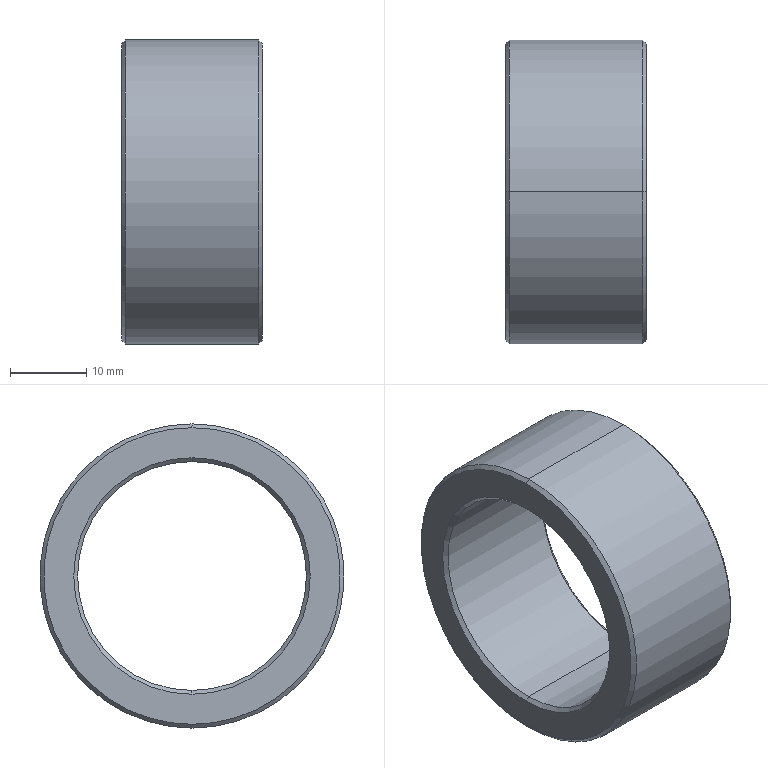Part | SolidWorks | features Chamfer 1, Extrusion 1 | 1 solid | 14 faces | box 18.5 x 40 x 40 mm | volume 10029 mm3 | cone 8 | cylinder 4 | plane 2 | commonest cylinder face diameters 30.1 x2 40 x2
STEP:
#1=CARTESIAN_POINT('',(18.5,0.,-19.5));
#2=VERTEX_POINT('',#1);
#3=CARTESIAN_POINT('',(18.5,0.,19.5));
#4=VERTEX_POINT('',#3);
#5=CARTESIAN_POINT('',(18.5,0.,0.));
#6=DIRECTION('',(1.,0.,0.));
#7=DIRECTION('',(0.,0.,-1.));
#8=AXIS2_PLACEMENT_3D('',#5,#6,#7);
#9=CIRCLE('',#8,19.5);
#10=EDGE_CURVE('',#2,#4,#9,.T.);
#11=ORIENTED_EDGE('',*,*,#10,.F.);
#12=CARTESIAN_POINT('',(18.,0.,-20.));
#13=VERTEX_POINT('',#12);
#14=CARTESIAN_POINT('',(18.5,0.,-19.5));
#15=DIRECTION('',(-0.7071,0.,-0.7071));
#16=VECTOR('',#15,1000.);
#17=LINE('',#14,#16);
#18=EDGE_CURVE('',#2,#13,#17,.T.);
#19=ORIENTED_EDGE('',*,*,#18,.T.);
#20=CARTESIAN_POINT('',(18.,0.,20.));
#21=VERTEX_POINT('',#20);
#22=CARTESIAN_POINT('',(18.,0.,0.));
#23=DIRECTION('',(-1.,0.,0.));
#24=DIRECTION('',(0.,0.,-1.));
#25=AXIS2_PLACEMENT_3D('',#22,#23,#24);
#26=CIRCLE('',#25,20.);
#27=EDGE_CURVE('',#21,#13,#26,.T.);
#28=ORIENTED_EDGE('',*,*,#27,.F.);
#29=CARTESIAN_POINT('',(18.5,0.,19.5));
#30=DIRECTION('',(-0.7071,0.,0.7071));
#31=VECTOR('',#30,1000.);
#32=LINE('',#29,#31);
#33=EDGE_CURVE('',#4,#21,#32,.T.);
#34=ORIENTED_EDGE('',*,*,#33,.F.);
#35=EDGE_LOOP('',(#11,#19,#28,#34));
#36=FACE_OUTER_BOUND('',#35,.T.);
#37=CARTESIAN_POINT('',(18.5,0.,0.));
#38=DIRECTION('',(-1.,0.,0.));
#39=DIRECTION('',(0.,0.,1.));
#40=AXIS2_PLACEMENT_3D('',#37,#38,#39);
#41=CONICAL_SURFACE('',#40,19.5,0.7854);
#42=ADVANCED_FACE('',(#36),#41,.T.);
#43=CARTESIAN_POINT('',(0.,0.,19.5));
#44=VERTEX_POINT('',#43);
#45=CARTESIAN_POINT('',(0.,0.,-19.5));
#46=VERTEX_POINT('',#45);
#47=CARTESIAN_POINT('',(0.,0.,0.));
#48=DIRECTION('',(-1.,0.,0.));
#49=DIRECTION('',(0.,0.,-1.));
#50=AXIS2_PLACEMENT_3D('',#47,#48,#49);
#51=CIRCLE('',#50,19.5);
#52=EDGE_CURVE('',#44,#46,#51,.T.);
#53=ORIENTED_EDGE('',*,*,#52,.F.);
#54=CARTESIAN_POINT('',(0.5,0.,20.));
#55=VERTEX_POINT('',#54);
#56=CARTESIAN_POINT('',(0.5,0.,20.));
#57=DIRECTION('',(0.7071,0.,0.7071));
#58=VECTOR('',#57,1000.);
#59=LINE('',#56,#58);
#60=EDGE_CURVE('',#44,#55,#59,.T.);
#61=ORIENTED_EDGE('',*,*,#60,.T.);
#62=CARTESIAN_POINT('',(0.5,0.,-20.));
#63=VERTEX_POINT('',#62);
#64=CARTESIAN_POINT('',(0.5,0.,0.));
#65=DIRECTION('',(1.,0.,0.));
#66=DIRECTION('',(0.,0.,-1.));
#67=AXIS2_PLACEMENT_3D('',#64,#65,#66);
#68=CIRCLE('',#67,20.);
#69=EDGE_CURVE('',#63,#55,#68,.T.);
#70=ORIENTED_EDGE('',*,*,#69,.F.);
#71=CARTESIAN_POINT('',(0.5,0.,-20.));
#72=DIRECTION('',(0.7071,0.,-0.7071));
#73=VECTOR('',#72,1000.);
#74=LINE('',#71,#73);
#75=EDGE_CURVE('',#46,#63,#74,.T.);
#76=ORIENTED_EDGE('',*,*,#75,.F.);
#77=EDGE_LOOP('',(#53,#61,#70,#76));
#78=FACE_OUTER_BOUND('',#77,.T.);
#79=CARTESIAN_POINT('',(0.5,0.,0.));
#80=DIRECTION('',(1.,0.,0.));
#81=DIRECTION('',(0.,0.,-1.));
#82=AXIS2_PLACEMENT_3D('',#79,#80,#81);
#83=CONICAL_SURFACE('',#82,20.,0.7854);
#84=ADVANCED_FACE('',(#78),#83,.T.);
#85=CARTESIAN_POINT('',(18.,0.,15.05));
#86=VERTEX_POINT('',#85);
#87=CARTESIAN_POINT('',(18.,0.,-15.05));
#88=VERTEX_POINT('',#87);
#89=CARTESIAN_POINT('',(18.,0.,0.));
#90=DIRECTION('',(1.,0.,0.));
#91=DIRECTION('',(0.,0.,-1.));
#92=AXIS2_PLACEMENT_3D('',#89,#90,#91);
#93=CIRCLE('',#92,15.05);
#94=EDGE_CURVE('',#86,#88,#93,.T.);
#95=ORIENTED_EDGE('',*,*,#94,.F.);
#96=CARTESIAN_POINT('',(18.5,0.,15.55));
#97=VERTEX_POINT('',#96);
#98=CARTESIAN_POINT('',(18.,0.,15.05));
#99=DIRECTION('',(0.7071,0.,0.7071));
#100=VECTOR('',#99,1000.);
#101=LINE('',#98,#100);
#102=EDGE_CURVE('',#86,#97,#101,.T.);
#103=ORIENTED_EDGE('',*,*,#102,.T.);
#104=CARTESIAN_POINT('',(18.5,0.,-15.55));
#105=VERTEX_POINT('',#104);
#106=CARTESIAN_POINT('',(18.5,0.,0.));
#107=DIRECTION('',(-1.,0.,0.));
#108=DIRECTION('',(0.,0.,-1.));
#109=AXIS2_PLACEMENT_3D('',#106,#107,#108);
#110=CIRCLE('',#109,15.55);
#111=EDGE_CURVE('',#105,#97,#110,.T.);
#112=ORIENTED_EDGE('',*,*,#111,.F.);
#113=CARTESIAN_POINT('',(18.,0.,-15.05));
#114=DIRECTION('',(0.7071,0.,-0.7071));
#115=VECTOR('',#114,1000.);
#116=LINE('',#113,#115);
#117=EDGE_CURVE('',#88,#105,#116,.T.);
#118=ORIENTED_EDGE('',*,*,#117,.F.);
#119=EDGE_LOOP('',(#95,#103,#112,#118));
#120=FACE_OUTER_BOUND('',#119,.T.);
#121=CARTESIAN_POINT('',(18.,0.,0.));
#122=DIRECTION('',(1.,0.,0.));
#123=DIRECTION('',(0.,0.,-1.));
#124=AXIS2_PLACEMENT_3D('',#121,#122,#123);
#125=CONICAL_SURFACE('',#124,15.05,0.7854);
#126=ADVANCED_FACE('',(#120),#125,.F.);
#127=CARTESIAN_POINT('',(0.5,0.,-15.05));
#128=VERTEX_POINT('',#127);
#129=CARTESIAN_POINT('',(0.5,0.,15.05));
#130=VERTEX_POINT('',#129);
#131=CARTESIAN_POINT('',(0.5,0.,0.));
#132=DIRECTION('',(-1.,0.,0.));
#133=DIRECTION('',(0.,0.,-1.));
#134=AXIS2_PLACEMENT_3D('',#131,#132,#133);
#135=CIRCLE('',#134,15.05);
#136=EDGE_CURVE('',#128,#130,#135,.T.);
#137=ORIENTED_EDGE('',*,*,#136,.F.);
#138=CARTESIAN_POINT('',(0.,0.,-15.55));
#139=VERTEX_POINT('',#138);
#140=CARTESIAN_POINT('',(0.,0.,-15.55));
#141=DIRECTION('',(-0.7071,0.,-0.7071));
#142=VECTOR('',#141,1000.);
#143=LINE('',#140,#142);
#144=EDGE_CURVE('',#128,#139,#143,.T.);
#145=ORIENTED_EDGE('',*,*,#144,.T.);
#146=CARTESIAN_POINT('',(0.,0.,15.55));
#147=VERTEX_POINT('',#146);
#148=CARTESIAN_POINT('',(0.,0.,0.));
#149=DIRECTION('',(1.,0.,0.));
#150=DIRECTION('',(0.,0.,-1.));
#151=AXIS2_PLACEMENT_3D('',#148,#149,#150);
#152=CIRCLE('',#151,15.55);
#153=EDGE_CURVE('',#147,#139,#152,.T.);
#154=ORIENTED_EDGE('',*,*,#153,.F.);
#155=CARTESIAN_POINT('',(0.,0.,15.55));
#156=DIRECTION('',(-0.7071,0.,0.7071));
#157=VECTOR('',#156,1000.);
#158=LINE('',#155,#157);
#159=EDGE_CURVE('',#130,#147,#158,.T.);
#160=ORIENTED_EDGE('',*,*,#159,.F.);
#161=EDGE_LOOP('',(#137,#145,#154,#160));
#162=FACE_OUTER_BOUND('',#161,.T.);
#163=CARTESIAN_POINT('',(0.,0.,0.));
#164=DIRECTION('',(-1.,0.,0.));
#165=DIRECTION('',(0.,0.,1.));
#166=AXIS2_PLACEMENT_3D('',#163,#164,#165);
#167=CONICAL_SURFACE('',#166,15.55,0.7854);
#168=ADVANCED_FACE('',(#162),#167,.F.);
#169=ORIENTED_EDGE('',*,*,#94,.T.);
#170=CARTESIAN_POINT('',(18.5,0.,-15.05));
#171=DIRECTION('',(-1.,0.,0.));
#172=VECTOR('',#171,1000.);
#173=LINE('',#170,#172);
#174=EDGE_CURVE('',#88,#128,#173,.T.);
#175=ORIENTED_EDGE('',*,*,#174,.T.);
#176=ORIENTED_EDGE('',*,*,#136,.T.);
#177=CARTESIAN_POINT('',(18.5,0.,15.05));
#178=DIRECTION('',(-1.,0.,0.));
#179=VECTOR('',#178,1000.);
#180=LINE('',#177,#179);
#181=EDGE_CURVE('',#86,#130,#180,.T.);
#182=ORIENTED_EDGE('',*,*,#181,.F.);
#183=EDGE_LOOP('',(#169,#175,#176,#182));
#184=FACE_OUTER_BOUND('',#183,.T.);
#185=CARTESIAN_POINT('',(18.5,0.,0.));
#186=DIRECTION('',(-1.,0.,0.));
#187=DIRECTION('',(0.,0.,1.));
#188=AXIS2_PLACEMENT_3D('',#185,#186,#187);
#189=CYLINDRICAL_SURFACE('',#188,15.05);
#190=ADVANCED_FACE('',(#184),#189,.F.);
#191=ORIENTED_EDGE('',*,*,#27,.T.);
#192=CARTESIAN_POINT('',(18.5,0.,-20.));
#193=DIRECTION('',(-1.,0.,0.));
#194=VECTOR('',#193,1000.);
#195=LINE('',#192,#194);
#196=EDGE_CURVE('',#13,#63,#195,.T.);
#197=ORIENTED_EDGE('',*,*,#196,.T.);
#198=ORIENTED_EDGE('',*,*,#69,.T.);
#199=CARTESIAN_POINT('',(18.5,0.,20.));
#200=DIRECTION('',(-1.,0.,0.));
#201=VECTOR('',#200,1000.);
#202=LINE('',#199,#201);
#203=EDGE_CURVE('',#21,#55,#202,.T.);
#204=ORIENTED_EDGE('',*,*,#203,.F.);
#205=EDGE_LOOP('',(#191,#197,#198,#204));
#206=FACE_OUTER_BOUND('',#205,.T.);
#207=CARTESIAN_POINT('',(18.5,0.,0.));
#208=DIRECTION('',(-1.,0.,0.));
#209=DIRECTION('',(0.,0.,1.));
#210=AXIS2_PLACEMENT_3D('',#207,#208,#209);
#211=CYLINDRICAL_SURFACE('',#210,20.);
#212=ADVANCED_FACE('',(#206),#211,.T.);
#213=ORIENTED_EDGE('',*,*,#111,.T.);
#214=CARTESIAN_POINT('',(18.5,0.,0.));
#215=DIRECTION('',(-1.,0.,0.));
#216=DIRECTION('',(0.,0.,-1.));
#217=AXIS2_PLACEMENT_3D('',#214,#215,#216);
#218=CIRCLE('',#217,15.55);
#219=EDGE_CURVE('',#97,#105,#218,.T.);
#220=ORIENTED_EDGE('',*,*,#219,.T.);
#221=EDGE_LOOP('',(#213,#220));
#222=FACE_BOUND('',#221,.T.);
#223=CARTESIAN_POINT('',(18.5,0.,0.));
#224=DIRECTION('',(1.,0.,0.));
#225=DIRECTION('',(0.,0.,-1.));
#226=AXIS2_PLACEMENT_3D('',#223,#224,#225);
#227=CIRCLE('',#226,19.5);
#228=EDGE_CURVE('',#4,#2,#227,.T.);
#229=ORIENTED_EDGE('',*,*,#228,.T.);
#230=ORIENTED_EDGE('',*,*,#10,.T.);
#231=EDGE_LOOP('',(#229,#230));
#232=FACE_OUTER_BOUND('',#231,.T.);
#233=CARTESIAN_POINT('',(18.5,0.,0.));
#234=DIRECTION('',(1.,0.,0.));
#235=DIRECTION('',(0.,0.,-1.));
#236=AXIS2_PLACEMENT_3D('',#233,#234,#235);
#237=PLANE('',#236);
#238=ADVANCED_FACE('',(#222,#232),#237,.T.);
#239=ORIENTED_EDGE('',*,*,#153,.T.);
#240=CARTESIAN_POINT('',(0.,0.,0.));
#241=DIRECTION('',(1.,0.,0.));
#242=DIRECTION('',(0.,0.,-1.));
#243=AXIS2_PLACEMENT_3D('',#240,#241,#242);
#244=CIRCLE('',#243,15.55);
#245=EDGE_CURVE('',#139,#147,#244,.T.);
#246=ORIENTED_EDGE('',*,*,#245,.T.);
#247=EDGE_LOOP('',(#239,#246));
#248=FACE_BOUND('',#247,.T.);
#249=CARTESIAN_POINT('',(0.,0.,0.));
#250=DIRECTION('',(-1.,0.,0.));
#251=DIRECTION('',(0.,0.,-1.));
#252=AXIS2_PLACEMENT_3D('',#249,#250,#251);
#253=CIRCLE('',#252,19.5);
#254=EDGE_CURVE('',#46,#44,#253,.T.);
#255=ORIENTED_EDGE('',*,*,#254,.T.);
#256=ORIENTED_EDGE('',*,*,#52,.T.);
#257=EDGE_LOOP('',(#255,#256));
#258=FACE_OUTER_BOUND('',#257,.T.);
#259=CARTESIAN_POINT('',(0.,0.,0.));
#260=DIRECTION('',(1.,0.,0.));
#261=DIRECTION('',(0.,0.,-1.));
#262=AXIS2_PLACEMENT_3D('',#259,#260,#261);
#263=PLANE('',#262);
#264=ADVANCED_FACE('',(#248,#258),#263,.F.);
#265=ORIENTED_EDGE('',*,*,#196,.F.);
#266=CARTESIAN_POINT('',(18.,0.,0.));
#267=DIRECTION('',(-1.,0.,0.));
#268=DIRECTION('',(0.,0.,-1.));
#269=AXIS2_PLACEMENT_3D('',#266,#267,#268);
#270=CIRCLE('',#269,20.);
#271=EDGE_CURVE('',#13,#21,#270,.T.);
#272=ORIENTED_EDGE('',*,*,#271,.T.);
#273=ORIENTED_EDGE('',*,*,#203,.T.);
#274=CARTESIAN_POINT('',(0.5,0.,0.));
#275=DIRECTION('',(1.,0.,0.));
#276=DIRECTION('',(0.,0.,-1.));
#277=AXIS2_PLACEMENT_3D('',#274,#275,#276);
#278=CIRCLE('',#277,20.);
#279=EDGE_CURVE('',#55,#63,#278,.T.);
#280=ORIENTED_EDGE('',*,*,#279,.T.);
#281=EDGE_LOOP('',(#265,#272,#273,#280));
#282=FACE_OUTER_BOUND('',#281,.T.);
#283=CARTESIAN_POINT('',(18.5,0.,0.));
#284=DIRECTION('',(-1.,0.,0.));
#285=DIRECTION('',(0.,0.,1.));
#286=AXIS2_PLACEMENT_3D('',#283,#284,#285);
#287=CYLINDRICAL_SURFACE('',#286,20.);
#288=ADVANCED_FACE('',(#282),#287,.T.);
#289=ORIENTED_EDGE('',*,*,#174,.F.);
#290=CARTESIAN_POINT('',(18.,0.,0.));
#291=DIRECTION('',(1.,0.,0.));
#292=DIRECTION('',(0.,0.,-1.));
#293=AXIS2_PLACEMENT_3D('',#290,#291,#292);
#294=CIRCLE('',#293,15.05);
#295=EDGE_CURVE('',#88,#86,#294,.T.);
#296=ORIENTED_EDGE('',*,*,#295,.T.);
#297=ORIENTED_EDGE('',*,*,#181,.T.);
#298=CARTESIAN_POINT('',(0.5,0.,0.));
#299=DIRECTION('',(-1.,0.,0.));
#300=DIRECTION('',(0.,0.,-1.));
#301=AXIS2_PLACEMENT_3D('',#298,#299,#300);
#302=CIRCLE('',#301,15.05);
#303=EDGE_CURVE('',#130,#128,#302,.T.);
#304=ORIENTED_EDGE('',*,*,#303,.T.);
#305=EDGE_LOOP('',(#289,#296,#297,#304));
#306=FACE_OUTER_BOUND('',#305,.T.);
#307=CARTESIAN_POINT('',(18.5,0.,0.));
#308=DIRECTION('',(-1.,0.,0.));
#309=DIRECTION('',(0.,0.,1.));
#310=AXIS2_PLACEMENT_3D('',#307,#308,#309);
#311=CYLINDRICAL_SURFACE('',#310,15.05);
#312=ADVANCED_FACE('',(#306),#311,.F.);
#313=ORIENTED_EDGE('',*,*,#144,.F.);
#314=ORIENTED_EDGE('',*,*,#303,.F.);
#315=ORIENTED_EDGE('',*,*,#159,.T.);
#316=ORIENTED_EDGE('',*,*,#245,.F.);
#317=EDGE_LOOP('',(#313,#314,#315,#316));
#318=FACE_OUTER_BOUND('',#317,.T.);
#319=CARTESIAN_POINT('',(0.,0.,0.));
#320=DIRECTION('',(-1.,0.,0.));
#321=DIRECTION('',(0.,0.,1.));
#322=AXIS2_PLACEMENT_3D('',#319,#320,#321);
#323=CONICAL_SURFACE('',#322,15.55,0.7854);
#324=ADVANCED_FACE('',(#318),#323,.F.);
#325=ORIENTED_EDGE('',*,*,#102,.F.);
#326=ORIENTED_EDGE('',*,*,#295,.F.);
#327=ORIENTED_EDGE('',*,*,#117,.T.);
#328=ORIENTED_EDGE('',*,*,#219,.F.);
#329=EDGE_LOOP('',(#325,#326,#327,#328));
#330=FACE_OUTER_BOUND('',#329,.T.);
#331=CARTESIAN_POINT('',(18.,0.,0.));
#332=DIRECTION('',(1.,0.,0.));
#333=DIRECTION('',(0.,0.,-1.));
#334=AXIS2_PLACEMENT_3D('',#331,#332,#333);
#335=CONICAL_SURFACE('',#334,15.05,0.7854);
#336=ADVANCED_FACE('',(#330),#335,.F.);
#337=ORIENTED_EDGE('',*,*,#60,.F.);
#338=ORIENTED_EDGE('',*,*,#254,.F.);
#339=ORIENTED_EDGE('',*,*,#75,.T.);
#340=ORIENTED_EDGE('',*,*,#279,.F.);
#341=EDGE_LOOP('',(#337,#338,#339,#340));
#342=FACE_OUTER_BOUND('',#341,.T.);
#343=CARTESIAN_POINT('',(0.5,0.,0.));
#344=DIRECTION('',(1.,0.,0.));
#345=DIRECTION('',(0.,0.,-1.));
#346=AXIS2_PLACEMENT_3D('',#343,#344,#345);
#347=CONICAL_SURFACE('',#346,20.,0.7854);
#348=ADVANCED_FACE('',(#342),#347,.T.);
#349=ORIENTED_EDGE('',*,*,#18,.F.);
#350=ORIENTED_EDGE('',*,*,#228,.F.);
#351=ORIENTED_EDGE('',*,*,#33,.T.);
#352=ORIENTED_EDGE('',*,*,#271,.F.);
#353=EDGE_LOOP('',(#349,#350,#351,#352));
#354=FACE_OUTER_BOUND('',#353,.T.);
#355=CARTESIAN_POINT('',(18.5,0.,0.));
#356=DIRECTION('',(-1.,0.,0.));
#357=DIRECTION('',(0.,0.,1.));
#358=AXIS2_PLACEMENT_3D('',#355,#356,#357);
#359=CONICAL_SURFACE('',#358,19.5,0.7854);
#360=ADVANCED_FACE('',(#354),#359,.T.);
#361=CLOSED_SHELL('',(#42,#84,#126,#168,#190,#212,#238,#264,#288,#312,#324,#336,#348,#360));
#362=MANIFOLD_SOLID_BREP('',#361);
#363=CARTESIAN_POINT('',(0.,0.,0.));
#364=DIRECTION('',(0.,0.,1.));
#365=DIRECTION('',(1.,0.,0.));
#366=AXIS2_PLACEMENT_3D('',#363,#364,#365);
#367=(LENGTH_UNIT()NAMED_UNIT(*)SI_UNIT(.MILLI.,.METRE.));
#368=UNCERTAINTY_MEASURE_WITH_UNIT(LENGTH_MEASURE(0.00001),#367,'','');
#369=(NAMED_UNIT(*)PLANE_ANGLE_UNIT()SI_UNIT($,.RADIAN.));
#370=(NAMED_UNIT(*)SI_UNIT($,.STERADIAN.)SOLID_ANGLE_UNIT());
#371=(GEOMETRIC_REPRESENTATION_CONTEXT(3)GLOBAL_UNCERTAINTY_ASSIGNED_CONTEXT((#368))GLOBAL_UNIT_ASSIGNED_CONTEXT((#367,#369,#370))REPRESENTATION_CONTEXT('',''));
#372=ADVANCED_BREP_SHAPE_REPRESENTATION('',(#362,#366),#371);